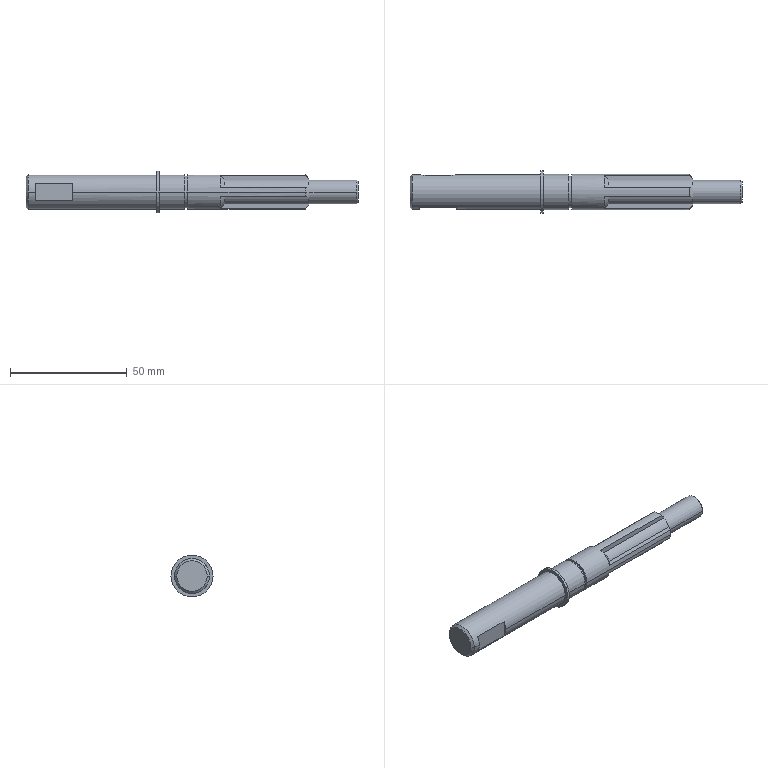Part | SolidWorks | features Chamfer 4, ICE 3, Revolution 1 | 1 solid | 52 faces | box 142 x 18 x 18 mm | volume 20860 mm3 | plane 21 | cylinder 18 | cone 13 | commonest cylinder face diameters 11 x4 15 x4 5 x2 10 x2 13.4 x2 14.964 x2